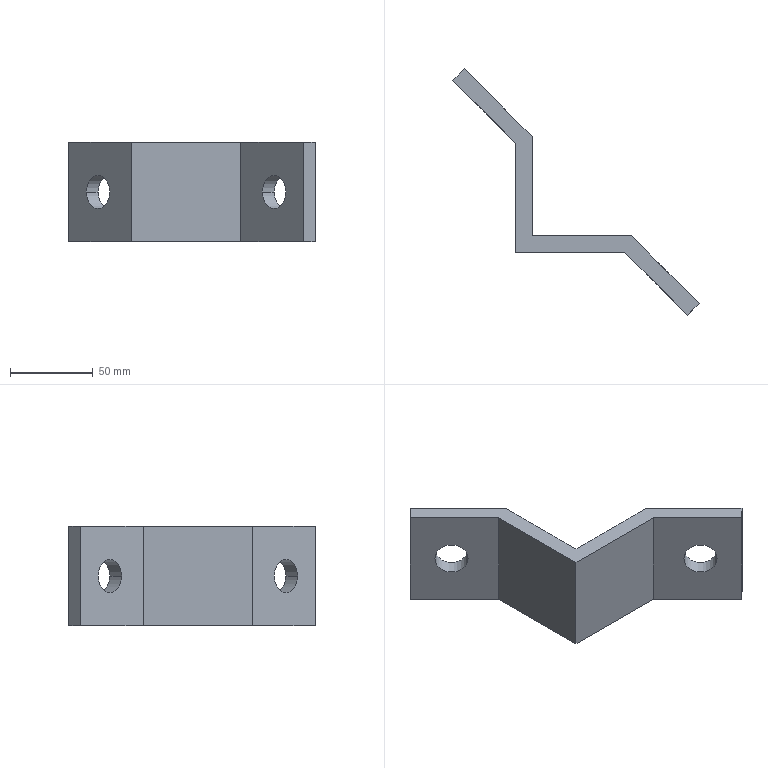Part | SolidWorks | features Cut 1, Extrusion 1, ICE 1 | 1 solid | 16 faces | box 148.492 x 148.492 x 60 mm | volume 135835 mm3 | plane 12 | cylinder 4 | commonest cylinder face diameters 20 x4
STEP:
#1=CARTESIAN_POINT('',(-30.104,90.104,30.));
#2=VERTEX_POINT('',#1);
#3=CARTESIAN_POINT('',(-15.962,75.962,30.));
#4=VERTEX_POINT('',#3);
#5=CARTESIAN_POINT('',(-23.033,83.033,30.));
#6=DIRECTION('',(-0.7071,-0.7071,0.));
#7=DIRECTION('',(0.7071,-0.7071,0.));
#8=AXIS2_PLACEMENT_3D('',#5,#6,#7);
#9=CIRCLE('',#8,10.);
#10=EDGE_CURVE('',#2,#4,#9,.T.);
#11=ORIENTED_EDGE('',*,*,#10,.F.);
#12=CARTESIAN_POINT('',(-37.175,83.033,30.));
#13=VERTEX_POINT('',#12);
#14=CARTESIAN_POINT('',(5.251,125.459,30.));
#15=DIRECTION('',(-0.7071,-0.7071,0.));
#16=VECTOR('',#15,1000.);
#17=LINE('',#14,#16);
#18=EDGE_CURVE('',#2,#13,#17,.T.);
#19=ORIENTED_EDGE('',*,*,#18,.T.);
#20=CARTESIAN_POINT('',(-23.033,68.891,30.));
#21=VERTEX_POINT('',#20);
#22=CARTESIAN_POINT('',(-30.104,75.962,30.));
#23=DIRECTION('',(-0.7071,-0.7071,0.));
#24=DIRECTION('',(0.7071,-0.7071,0.));
#25=AXIS2_PLACEMENT_3D('',#22,#23,#24);
#26=CIRCLE('',#25,10.);
#27=EDGE_CURVE('',#13,#21,#26,.T.);
#28=ORIENTED_EDGE('',*,*,#27,.T.);
#29=CARTESIAN_POINT('',(19.393,111.317,30.));
#30=DIRECTION('',(-0.7071,-0.7071,0.));
#31=VECTOR('',#30,1000.);
#32=LINE('',#29,#31);
#33=EDGE_CURVE('',#4,#21,#32,.T.);
#34=ORIENTED_EDGE('',*,*,#33,.F.);
#35=EDGE_LOOP('',(#11,#19,#28,#34));
#36=FACE_OUTER_BOUND('',#35,.T.);
#37=CARTESIAN_POINT('',(12.322,118.388,30.));
#38=DIRECTION('',(-0.7071,-0.7071,0.));
#39=DIRECTION('',(0.7071,-0.7071,0.));
#40=AXIS2_PLACEMENT_3D('',#37,#38,#39);
#41=CYLINDRICAL_SURFACE('',#40,10.);
#42=ADVANCED_FACE('',(#36),#41,.F.);
#43=CARTESIAN_POINT('',(75.962,-15.962,30.));
#44=VERTEX_POINT('',#43);
#45=CARTESIAN_POINT('',(90.104,-30.104,30.));
#46=VERTEX_POINT('',#45);
#47=CARTESIAN_POINT('',(83.033,-23.033,30.));
#48=DIRECTION('',(-0.7071,-0.7071,0.));
#49=DIRECTION('',(0.7071,-0.7071,0.));
#50=AXIS2_PLACEMENT_3D('',#47,#48,#49);
#51=CIRCLE('',#50,10.);
#52=EDGE_CURVE('',#44,#46,#51,.T.);
#53=ORIENTED_EDGE('',*,*,#52,.F.);
#54=CARTESIAN_POINT('',(68.891,-23.033,30.));
#55=VERTEX_POINT('',#54);
#56=CARTESIAN_POINT('',(111.317,19.393,30.));
#57=DIRECTION('',(-0.7071,-0.7071,0.));
#58=VECTOR('',#57,1000.);
#59=LINE('',#56,#58);
#60=EDGE_CURVE('',#44,#55,#59,.T.);
#61=ORIENTED_EDGE('',*,*,#60,.T.);
#62=CARTESIAN_POINT('',(83.033,-37.175,30.));
#63=VERTEX_POINT('',#62);
#64=CARTESIAN_POINT('',(75.962,-30.104,30.));
#65=DIRECTION('',(-0.7071,-0.7071,0.));
#66=DIRECTION('',(0.7071,-0.7071,0.));
#67=AXIS2_PLACEMENT_3D('',#64,#65,#66);
#68=CIRCLE('',#67,10.);
#69=EDGE_CURVE('',#55,#63,#68,.T.);
#70=ORIENTED_EDGE('',*,*,#69,.T.);
#71=CARTESIAN_POINT('',(125.459,5.251,30.));
#72=DIRECTION('',(-0.7071,-0.7071,0.));
#73=VECTOR('',#72,1000.);
#74=LINE('',#71,#73);
#75=EDGE_CURVE('',#46,#63,#74,.T.);
#76=ORIENTED_EDGE('',*,*,#75,.F.);
#77=EDGE_LOOP('',(#53,#61,#70,#76));
#78=FACE_OUTER_BOUND('',#77,.T.);
#79=CARTESIAN_POINT('',(118.388,12.322,30.));
#80=DIRECTION('',(-0.7071,-0.7071,0.));
#81=DIRECTION('',(0.7071,-0.7071,0.));
#82=AXIS2_PLACEMENT_3D('',#79,#80,#81);
#83=CYLINDRICAL_SURFACE('',#82,10.);
#84=ADVANCED_FACE('',(#78),#83,.F.);
#85=CARTESIAN_POINT('',(55.858,-10.,60.));
#86=VERTEX_POINT('',#85);
#87=CARTESIAN_POINT('',(55.858,-10.,0.));
#88=VERTEX_POINT('',#87);
#89=CARTESIAN_POINT('',(55.858,-10.,60.));
#90=DIRECTION('',(0.,0.,-1.));
#91=VECTOR('',#90,1000.);
#92=LINE('',#89,#91);
#93=EDGE_CURVE('',#86,#88,#92,.T.);
#94=ORIENTED_EDGE('',*,*,#93,.F.);
#95=CARTESIAN_POINT('',(-10.,-10.,60.));
#96=VERTEX_POINT('',#95);
#97=CARTESIAN_POINT('',(-10.,-10.,60.));
#98=DIRECTION('',(1.,0.,0.));
#99=VECTOR('',#98,1000.);
#100=LINE('',#97,#99);
#101=EDGE_CURVE('',#96,#86,#100,.T.);
#102=ORIENTED_EDGE('',*,*,#101,.F.);
#103=CARTESIAN_POINT('',(-10.,-10.,0.));
#104=VERTEX_POINT('',#103);
#105=CARTESIAN_POINT('',(-10.,-10.,60.));
#106=DIRECTION('',(0.,0.,-1.));
#107=VECTOR('',#106,1000.);
#108=LINE('',#105,#107);
#109=EDGE_CURVE('',#96,#104,#108,.T.);
#110=ORIENTED_EDGE('',*,*,#109,.T.);
#111=CARTESIAN_POINT('',(-10.,-10.,0.));
#112=DIRECTION('',(1.,0.,0.));
#113=VECTOR('',#112,1000.);
#114=LINE('',#111,#113);
#115=EDGE_CURVE('',#104,#88,#114,.T.);
#116=ORIENTED_EDGE('',*,*,#115,.T.);
#117=EDGE_LOOP('',(#94,#102,#110,#116));
#118=FACE_OUTER_BOUND('',#117,.T.);
#119=CARTESIAN_POINT('',(-10.,-10.,60.));
#120=DIRECTION('',(0.,1.,0.));
#121=DIRECTION('',(0.,0.,1.));
#122=AXIS2_PLACEMENT_3D('',#119,#120,#121);
#123=PLANE('',#122);
#124=ADVANCED_FACE('',(#118),#123,.F.);
#125=CARTESIAN_POINT('',(-10.,55.858,60.));
#126=VERTEX_POINT('',#125);
#127=CARTESIAN_POINT('',(-10.,55.858,0.));
#128=VERTEX_POINT('',#127);
#129=CARTESIAN_POINT('',(-10.,55.858,60.));
#130=DIRECTION('',(0.,0.,-1.));
#131=VECTOR('',#130,1000.);
#132=LINE('',#129,#131);
#133=EDGE_CURVE('',#126,#128,#132,.T.);
#134=ORIENTED_EDGE('',*,*,#133,.T.);
#135=CARTESIAN_POINT('',(-10.,60.,0.));
#136=DIRECTION('',(0.,-1.,0.));
#137=VECTOR('',#136,1000.);
#138=LINE('',#135,#137);
#139=EDGE_CURVE('',#128,#104,#138,.T.);
#140=ORIENTED_EDGE('',*,*,#139,.T.);
#141=ORIENTED_EDGE('',*,*,#109,.F.);
#142=CARTESIAN_POINT('',(-10.,60.,60.));
#143=DIRECTION('',(0.,-1.,0.));
#144=VECTOR('',#143,1000.);
#145=LINE('',#142,#144);
#146=EDGE_CURVE('',#126,#96,#145,.T.);
#147=ORIENTED_EDGE('',*,*,#146,.F.);
#148=EDGE_LOOP('',(#134,#140,#141,#147));
#149=FACE_OUTER_BOUND('',#148,.T.);
#150=CARTESIAN_POINT('',(-10.,60.,60.));
#151=DIRECTION('',(1.,0.,0.));
#152=DIRECTION('',(0.,1.,0.));
#153=AXIS2_PLACEMENT_3D('',#150,#151,#152);
#154=PLANE('',#153);
#155=ADVANCED_FACE('',(#149),#154,.F.);
#156=CARTESIAN_POINT('',(60.,0.,0.));
#157=VERTEX_POINT('',#156);
#158=CARTESIAN_POINT('',(0.,0.,0.));
#159=VERTEX_POINT('',#158);
#160=CARTESIAN_POINT('',(60.,0.,0.));
#161=DIRECTION('',(-1.,0.,0.));
#162=VECTOR('',#161,1000.);
#163=LINE('',#160,#162);
#164=EDGE_CURVE('',#157,#159,#163,.T.);
#165=ORIENTED_EDGE('',*,*,#164,.T.);
#166=CARTESIAN_POINT('',(0.,0.,60.));
#167=VERTEX_POINT('',#166);
#168=CARTESIAN_POINT('',(0.,0.,60.));
#169=DIRECTION('',(0.,0.,-1.));
#170=VECTOR('',#169,1000.);
#171=LINE('',#168,#170);
#172=EDGE_CURVE('',#167,#159,#171,.T.);
#173=ORIENTED_EDGE('',*,*,#172,.F.);
#174=CARTESIAN_POINT('',(60.,0.,60.));
#175=VERTEX_POINT('',#174);
#176=CARTESIAN_POINT('',(60.,0.,60.));
#177=DIRECTION('',(-1.,0.,0.));
#178=VECTOR('',#177,1000.);
#179=LINE('',#176,#178);
#180=EDGE_CURVE('',#175,#167,#179,.T.);
#181=ORIENTED_EDGE('',*,*,#180,.F.);
#182=CARTESIAN_POINT('',(60.,0.,60.));
#183=DIRECTION('',(0.,0.,-1.));
#184=VECTOR('',#183,1000.);
#185=LINE('',#182,#184);
#186=EDGE_CURVE('',#175,#157,#185,.T.);
#187=ORIENTED_EDGE('',*,*,#186,.T.);
#188=EDGE_LOOP('',(#165,#173,#181,#187));
#189=FACE_OUTER_BOUND('',#188,.T.);
#190=CARTESIAN_POINT('',(60.,0.,60.));
#191=DIRECTION('',(0.,-1.,0.));
#192=DIRECTION('',(1.,0.,0.));
#193=AXIS2_PLACEMENT_3D('',#190,#191,#192);
#194=PLANE('',#193);
#195=ADVANCED_FACE('',(#189),#194,.F.);
#196=CARTESIAN_POINT('',(0.,60.,0.));
#197=VERTEX_POINT('',#196);
#198=CARTESIAN_POINT('',(0.,0.,0.));
#199=DIRECTION('',(0.,1.,0.));
#200=VECTOR('',#199,1000.);
#201=LINE('',#198,#200);
#202=EDGE_CURVE('',#159,#197,#201,.T.);
#203=ORIENTED_EDGE('',*,*,#202,.T.);
#204=CARTESIAN_POINT('',(0.,60.,60.));
#205=VERTEX_POINT('',#204);
#206=CARTESIAN_POINT('',(0.,60.,60.));
#207=DIRECTION('',(0.,0.,-1.));
#208=VECTOR('',#207,1000.);
#209=LINE('',#206,#208);
#210=EDGE_CURVE('',#205,#197,#209,.T.);
#211=ORIENTED_EDGE('',*,*,#210,.F.);
#212=CARTESIAN_POINT('',(0.,0.,60.));
#213=DIRECTION('',(0.,1.,0.));
#214=VECTOR('',#213,1000.);
#215=LINE('',#212,#214);
#216=EDGE_CURVE('',#167,#205,#215,.T.);
#217=ORIENTED_EDGE('',*,*,#216,.F.);
#218=ORIENTED_EDGE('',*,*,#172,.T.);
#219=EDGE_LOOP('',(#203,#211,#217,#218));
#220=FACE_OUTER_BOUND('',#219,.T.);
#221=CARTESIAN_POINT('',(0.,0.,60.));
#222=DIRECTION('',(-1.,0.,0.));
#223=DIRECTION('',(0.,0.,1.));
#224=AXIS2_PLACEMENT_3D('',#221,#222,#223);
#225=PLANE('',#224);
#226=ADVANCED_FACE('',(#220),#225,.F.);
#227=CARTESIAN_POINT('',(100.711,-40.711,60.));
#228=VERTEX_POINT('',#227);
#229=CARTESIAN_POINT('',(60.,0.,60.));
#230=DIRECTION('',(-0.7071,0.7071,0.));
#231=VECTOR('',#230,1000.);
#232=LINE('',#229,#231);
#233=EDGE_CURVE('',#228,#175,#232,.T.);
#234=ORIENTED_EDGE('',*,*,#233,.T.);
#235=ORIENTED_EDGE('',*,*,#180,.T.);
#236=ORIENTED_EDGE('',*,*,#216,.T.);
#237=CARTESIAN_POINT('',(-40.711,100.711,60.));
#238=VERTEX_POINT('',#237);
#239=CARTESIAN_POINT('',(0.,60.,60.));
#240=DIRECTION('',(-0.7071,0.7071,0.));
#241=VECTOR('',#240,1000.);
#242=LINE('',#239,#241);
#243=EDGE_CURVE('',#205,#238,#242,.T.);
#244=ORIENTED_EDGE('',*,*,#243,.T.);
#245=CARTESIAN_POINT('',(-47.782,93.64,60.));
#246=VERTEX_POINT('',#245);
#247=CARTESIAN_POINT('',(-40.711,100.711,60.));
#248=DIRECTION('',(-0.7071,-0.7071,0.));
#249=VECTOR('',#248,1000.);
#250=LINE('',#247,#249);
#251=EDGE_CURVE('',#238,#246,#250,.T.);
#252=ORIENTED_EDGE('',*,*,#251,.T.);
#253=CARTESIAN_POINT('',(-47.782,93.64,60.));
#254=DIRECTION('',(0.7071,-0.7071,0.));
#255=VECTOR('',#254,1000.);
#256=LINE('',#253,#255);
#257=EDGE_CURVE('',#246,#126,#256,.T.);
#258=ORIENTED_EDGE('',*,*,#257,.T.);
#259=ORIENTED_EDGE('',*,*,#146,.T.);
#260=ORIENTED_EDGE('',*,*,#101,.T.);
#261=CARTESIAN_POINT('',(93.64,-47.782,60.));
#262=VERTEX_POINT('',#261);
#263=CARTESIAN_POINT('',(93.64,-47.782,60.));
#264=DIRECTION('',(0.7071,-0.7071,0.));
#265=VECTOR('',#264,1000.);
#266=LINE('',#263,#265);
#267=EDGE_CURVE('',#86,#262,#266,.T.);
#268=ORIENTED_EDGE('',*,*,#267,.T.);
#269=CARTESIAN_POINT('',(100.711,-40.711,60.));
#270=DIRECTION('',(0.7071,0.7071,0.));
#271=VECTOR('',#270,1000.);
#272=LINE('',#269,#271);
#273=EDGE_CURVE('',#262,#228,#272,.T.);
#274=ORIENTED_EDGE('',*,*,#273,.T.);
#275=EDGE_LOOP('',(#234,#235,#236,#244,#252,#258,#259,#260,#268,#274));
#276=FACE_OUTER_BOUND('',#275,.T.);
#277=CARTESIAN_POINT('',(0.,0.,60.));
#278=DIRECTION('',(0.,0.,-1.));
#279=DIRECTION('',(-1.,0.,0.));
#280=AXIS2_PLACEMENT_3D('',#277,#278,#279);
#281=PLANE('',#280);
#282=ADVANCED_FACE('',(#276),#281,.F.);
#283=ORIENTED_EDGE('',*,*,#164,.F.);
#284=CARTESIAN_POINT('',(100.711,-40.711,0.));
#285=VERTEX_POINT('',#284);
#286=CARTESIAN_POINT('',(60.,0.,0.));
#287=DIRECTION('',(-0.7071,0.7071,0.));
#288=VECTOR('',#287,1000.);
#289=LINE('',#286,#288);
#290=EDGE_CURVE('',#285,#157,#289,.T.);
#291=ORIENTED_EDGE('',*,*,#290,.F.);
#292=CARTESIAN_POINT('',(93.64,-47.782,0.));
#293=VERTEX_POINT('',#292);
#294=CARTESIAN_POINT('',(100.711,-40.711,0.));
#295=DIRECTION('',(0.7071,0.7071,0.));
#296=VECTOR('',#295,1000.);
#297=LINE('',#294,#296);
#298=EDGE_CURVE('',#293,#285,#297,.T.);
#299=ORIENTED_EDGE('',*,*,#298,.F.);
#300=CARTESIAN_POINT('',(93.64,-47.782,0.));
#301=DIRECTION('',(0.7071,-0.7071,0.));
#302=VECTOR('',#301,1000.);
#303=LINE('',#300,#302);
#304=EDGE_CURVE('',#88,#293,#303,.T.);
#305=ORIENTED_EDGE('',*,*,#304,.F.);
#306=ORIENTED_EDGE('',*,*,#115,.F.);
#307=ORIENTED_EDGE('',*,*,#139,.F.);
#308=CARTESIAN_POINT('',(-47.782,93.64,0.));
#309=VERTEX_POINT('',#308);
#310=CARTESIAN_POINT('',(-47.782,93.64,0.));
#311=DIRECTION('',(0.7071,-0.7071,0.));
#312=VECTOR('',#311,1000.);
#313=LINE('',#310,#312);
#314=EDGE_CURVE('',#309,#128,#313,.T.);
#315=ORIENTED_EDGE('',*,*,#314,.F.);
#316=CARTESIAN_POINT('',(-40.711,100.711,0.));
#317=VERTEX_POINT('',#316);
#318=CARTESIAN_POINT('',(-40.711,100.711,0.));
#319=DIRECTION('',(-0.7071,-0.7071,0.));
#320=VECTOR('',#319,1000.);
#321=LINE('',#318,#320);
#322=EDGE_CURVE('',#317,#309,#321,.T.);
#323=ORIENTED_EDGE('',*,*,#322,.F.);
#324=CARTESIAN_POINT('',(0.,60.,0.));
#325=DIRECTION('',(-0.7071,0.7071,0.));
#326=VECTOR('',#325,1000.);
#327=LINE('',#324,#326);
#328=EDGE_CURVE('',#197,#317,#327,.T.);
#329=ORIENTED_EDGE('',*,*,#328,.F.);
#330=ORIENTED_EDGE('',*,*,#202,.F.);
#331=EDGE_LOOP('',(#283,#291,#299,#305,#306,#307,#315,#323,#329,#330));
#332=FACE_OUTER_BOUND('',#331,.T.);
#333=CARTESIAN_POINT('',(0.,0.,0.));
#334=DIRECTION('',(0.,0.,-1.));
#335=DIRECTION('',(-1.,0.,0.));
#336=AXIS2_PLACEMENT_3D('',#333,#334,#335);
#337=PLANE('',#336);
#338=ADVANCED_FACE('',(#332),#337,.T.);
#339=CARTESIAN_POINT('',(-23.033,83.033,30.));
#340=DIRECTION('',(-0.7071,-0.7071,0.));
#341=DIRECTION('',(0.7071,-0.7071,0.));
#342=AXIS2_PLACEMENT_3D('',#339,#340,#341);
#343=CIRCLE('',#342,10.);
#344=EDGE_CURVE('',#4,#2,#343,.T.);
#345=ORIENTED_EDGE('',*,*,#344,.T.);
#346=ORIENTED_EDGE('',*,*,#10,.T.);
#347=EDGE_LOOP('',(#345,#346));
#348=FACE_BOUND('',#347,.T.);
#349=ORIENTED_EDGE('',*,*,#328,.T.);
#350=CARTESIAN_POINT('',(-40.711,100.711,60.));
#351=DIRECTION('',(0.,0.,-1.));
#352=VECTOR('',#351,1000.);
#353=LINE('',#350,#352);
#354=EDGE_CURVE('',#238,#317,#353,.T.);
#355=ORIENTED_EDGE('',*,*,#354,.F.);
#356=ORIENTED_EDGE('',*,*,#243,.F.);
#357=ORIENTED_EDGE('',*,*,#210,.T.);
#358=EDGE_LOOP('',(#349,#355,#356,#357));
#359=FACE_OUTER_BOUND('',#358,.T.);
#360=CARTESIAN_POINT('',(0.,60.,60.));
#361=DIRECTION('',(-0.7071,-0.7071,0.));
#362=DIRECTION('',(0.7071,-0.7071,0.));
#363=AXIS2_PLACEMENT_3D('',#360,#361,#362);
#364=PLANE('',#363);
#365=ADVANCED_FACE('',(#348,#359),#364,.F.);
#366=ORIENTED_EDGE('',*,*,#322,.T.);
#367=CARTESIAN_POINT('',(-47.782,93.64,60.));
#368=DIRECTION('',(0.,0.,-1.));
#369=VECTOR('',#368,1000.);
#370=LINE('',#367,#369);
#371=EDGE_CURVE('',#246,#309,#370,.T.);
#372=ORIENTED_EDGE('',*,*,#371,.F.);
#373=ORIENTED_EDGE('',*,*,#251,.F.);
#374=ORIENTED_EDGE('',*,*,#354,.T.);
#375=EDGE_LOOP('',(#366,#372,#373,#374));
#376=FACE_OUTER_BOUND('',#375,.T.);
#377=CARTESIAN_POINT('',(-40.711,100.711,60.));
#378=DIRECTION('',(0.7071,-0.7071,0.));
#379=DIRECTION('',(0.7071,0.7071,0.));
#380=AXIS2_PLACEMENT_3D('',#377,#378,#379);
#381=PLANE('',#380);
#382=ADVANCED_FACE('',(#376),#381,.F.);
#383=CARTESIAN_POINT('',(-30.104,75.962,30.));
#384=DIRECTION('',(-0.7071,-0.7071,0.));
#385=DIRECTION('',(0.7071,-0.7071,0.));
#386=AXIS2_PLACEMENT_3D('',#383,#384,#385);
#387=CIRCLE('',#386,10.);
#388=EDGE_CURVE('',#21,#13,#387,.T.);
#389=ORIENTED_EDGE('',*,*,#388,.F.);
#390=ORIENTED_EDGE('',*,*,#27,.F.);
#391=EDGE_LOOP('',(#389,#390));
#392=FACE_BOUND('',#391,.T.);
#393=ORIENTED_EDGE('',*,*,#314,.T.);
#394=ORIENTED_EDGE('',*,*,#133,.F.);
#395=ORIENTED_EDGE('',*,*,#257,.F.);
#396=ORIENTED_EDGE('',*,*,#371,.T.);
#397=EDGE_LOOP('',(#393,#394,#395,#396));
#398=FACE_OUTER_BOUND('',#397,.T.);
#399=CARTESIAN_POINT('',(-47.782,93.64,60.));
#400=DIRECTION('',(0.7071,0.7071,0.));
#401=DIRECTION('',(-0.7071,0.7071,0.));
#402=AXIS2_PLACEMENT_3D('',#399,#400,#401);
#403=PLANE('',#402);
#404=ADVANCED_FACE('',(#392,#398),#403,.F.);
#405=CARTESIAN_POINT('',(75.962,-30.104,30.));
#406=DIRECTION('',(-0.7071,-0.7071,0.));
#407=DIRECTION('',(0.7071,-0.7071,0.));
#408=AXIS2_PLACEMENT_3D('',#405,#406,#407);
#409=CIRCLE('',#408,10.);
#410=EDGE_CURVE('',#63,#55,#409,.T.);
#411=ORIENTED_EDGE('',*,*,#410,.F.);
#412=ORIENTED_EDGE('',*,*,#69,.F.);
#413=EDGE_LOOP('',(#411,#412));
#414=FACE_BOUND('',#413,.T.);
#415=ORIENTED_EDGE('',*,*,#304,.T.);
#416=CARTESIAN_POINT('',(93.64,-47.782,60.));
#417=DIRECTION('',(0.,0.,-1.));
#418=VECTOR('',#417,1000.);
#419=LINE('',#416,#418);
#420=EDGE_CURVE('',#262,#293,#419,.T.);
#421=ORIENTED_EDGE('',*,*,#420,.F.);
#422=ORIENTED_EDGE('',*,*,#267,.F.);
#423=ORIENTED_EDGE('',*,*,#93,.T.);
#424=EDGE_LOOP('',(#415,#421,#422,#423));
#425=FACE_OUTER_BOUND('',#424,.T.);
#426=CARTESIAN_POINT('',(93.64,-47.782,60.));
#427=DIRECTION('',(0.7071,0.7071,0.));
#428=DIRECTION('',(-0.7071,0.7071,0.));
#429=AXIS2_PLACEMENT_3D('',#426,#427,#428);
#430=PLANE('',#429);
#431=ADVANCED_FACE('',(#414,#425),#430,.F.);
#432=ORIENTED_EDGE('',*,*,#298,.T.);
#433=CARTESIAN_POINT('',(100.711,-40.711,60.));
#434=DIRECTION('',(0.,0.,-1.));
#435=VECTOR('',#434,1000.);
#436=LINE('',#433,#435);
#437=EDGE_CURVE('',#228,#285,#436,.T.);
#438=ORIENTED_EDGE('',*,*,#437,.F.);
#439=ORIENTED_EDGE('',*,*,#273,.F.);
#440=ORIENTED_EDGE('',*,*,#420,.T.);
#441=EDGE_LOOP('',(#432,#438,#439,#440));
#442=FACE_OUTER_BOUND('',#441,.T.);
#443=CARTESIAN_POINT('',(100.711,-40.711,60.));
#444=DIRECTION('',(-0.7071,0.7071,0.));
#445=DIRECTION('',(-0.7071,-0.7071,0.));
#446=AXIS2_PLACEMENT_3D('',#443,#444,#445);
#447=PLANE('',#446);
#448=ADVANCED_FACE('',(#442),#447,.F.);
#449=CARTESIAN_POINT('',(83.033,-23.033,30.));
#450=DIRECTION('',(-0.7071,-0.7071,0.));
#451=DIRECTION('',(0.7071,-0.7071,0.));
#452=AXIS2_PLACEMENT_3D('',#449,#450,#451);
#453=CIRCLE('',#452,10.);
#454=EDGE_CURVE('',#46,#44,#453,.T.);
#455=ORIENTED_EDGE('',*,*,#454,.T.);
#456=ORIENTED_EDGE('',*,*,#52,.T.);
#457=EDGE_LOOP('',(#455,#456));
#458=FACE_BOUND('',#457,.T.);
#459=ORIENTED_EDGE('',*,*,#290,.T.);
#460=ORIENTED_EDGE('',*,*,#186,.F.);
#461=ORIENTED_EDGE('',*,*,#233,.F.);
#462=ORIENTED_EDGE('',*,*,#437,.T.);
#463=EDGE_LOOP('',(#459,#460,#461,#462));
#464=FACE_OUTER_BOUND('',#463,.T.);
#465=CARTESIAN_POINT('',(60.,0.,60.));
#466=DIRECTION('',(-0.7071,-0.7071,0.));
#467=DIRECTION('',(0.7071,-0.7071,0.));
#468=AXIS2_PLACEMENT_3D('',#465,#466,#467);
#469=PLANE('',#468);
#470=ADVANCED_FACE('',(#458,#464),#469,.F.);
#471=ORIENTED_EDGE('',*,*,#60,.F.);
#472=ORIENTED_EDGE('',*,*,#454,.F.);
#473=ORIENTED_EDGE('',*,*,#75,.T.);
#474=ORIENTED_EDGE('',*,*,#410,.T.);
#475=EDGE_LOOP('',(#471,#472,#473,#474));
#476=FACE_OUTER_BOUND('',#475,.T.);
#477=CARTESIAN_POINT('',(118.388,12.322,30.));
#478=DIRECTION('',(-0.7071,-0.7071,0.));
#479=DIRECTION('',(0.7071,-0.7071,0.));
#480=AXIS2_PLACEMENT_3D('',#477,#478,#479);
#481=CYLINDRICAL_SURFACE('',#480,10.);
#482=ADVANCED_FACE('',(#476),#481,.F.);
#483=ORIENTED_EDGE('',*,*,#18,.F.);
#484=ORIENTED_EDGE('',*,*,#344,.F.);
#485=ORIENTED_EDGE('',*,*,#33,.T.);
#486=ORIENTED_EDGE('',*,*,#388,.T.);
#487=EDGE_LOOP('',(#483,#484,#485,#486));
#488=FACE_OUTER_BOUND('',#487,.T.);
#489=CARTESIAN_POINT('',(12.322,118.388,30.));
#490=DIRECTION('',(-0.7071,-0.7071,0.));
#491=DIRECTION('',(0.7071,-0.7071,0.));
#492=AXIS2_PLACEMENT_3D('',#489,#490,#491);
#493=CYLINDRICAL_SURFACE('',#492,10.);
#494=ADVANCED_FACE('',(#488),#493,.F.);
#495=CLOSED_SHELL('',(#42,#84,#124,#155,#195,#226,#282,#338,#365,#382,#404,#431,#448,#470,#482,#494));
#496=MANIFOLD_SOLID_BREP('',#495);
#497=CARTESIAN_POINT('',(0.,0.,0.));
#498=DIRECTION('',(0.,0.,1.));
#499=DIRECTION('',(1.,0.,0.));
#500=AXIS2_PLACEMENT_3D('',#497,#498,#499);
#501=(LENGTH_UNIT()NAMED_UNIT(*)SI_UNIT(.MILLI.,.METRE.));
#502=UNCERTAINTY_MEASURE_WITH_UNIT(LENGTH_MEASURE(0.00001),#501,'','');
#503=(NAMED_UNIT(*)PLANE_ANGLE_UNIT()SI_UNIT($,.RADIAN.));
#504=(NAMED_UNIT(*)SI_UNIT($,.STERADIAN.)SOLID_ANGLE_UNIT());
#505=(GEOMETRIC_REPRESENTATION_CONTEXT(3)GLOBAL_UNCERTAINTY_ASSIGNED_CONTEXT((#502))GLOBAL_UNIT_ASSIGNED_CONTEXT((#501,#503,#504))REPRESENTATION_CONTEXT('',''));
#506=ADVANCED_BREP_SHAPE_REPRESENTATION('',(#496,#500),#505);